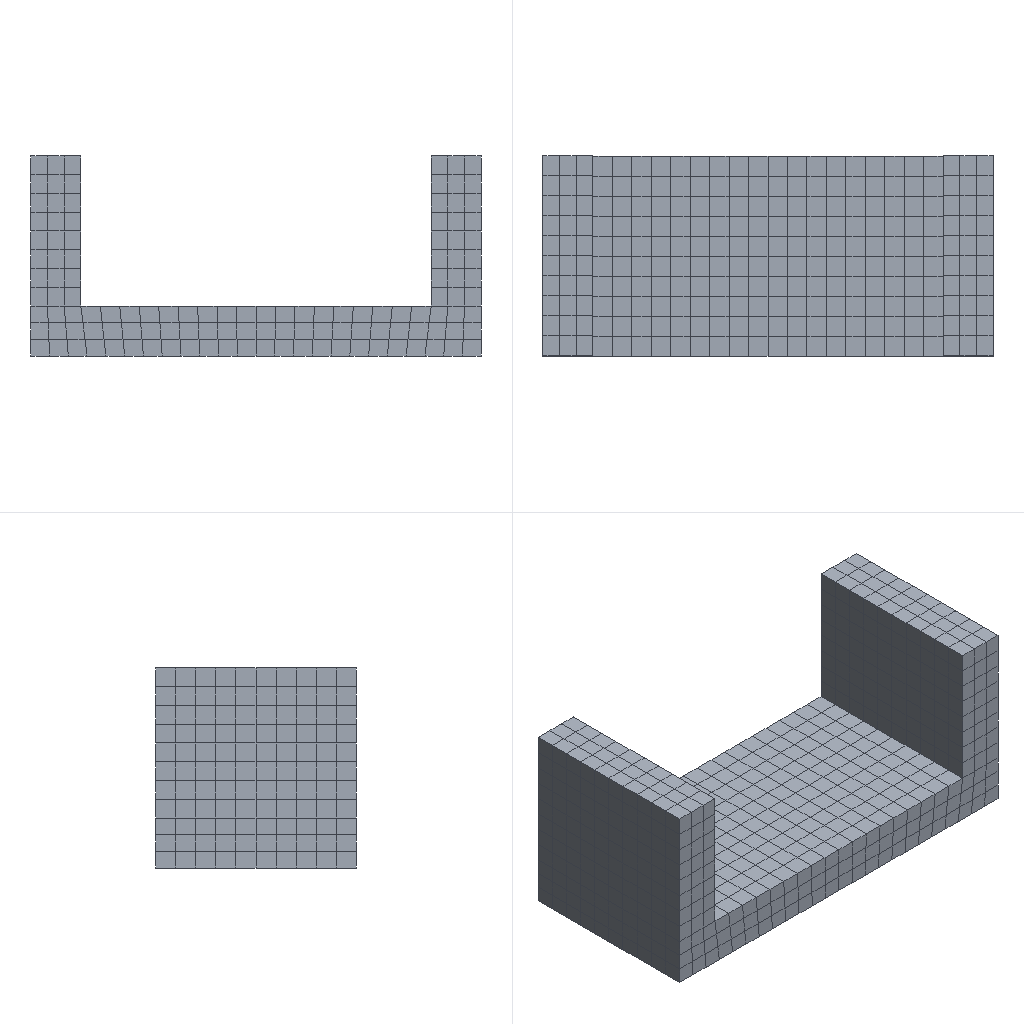Simulation study | abaqus
Notes in the study folder:
*Spring, elset=Springs/Dashpots-1-spring
1,1
 0.219E+06
*Element, type=Spring2, elset=Springs/Dashpots-1-spring
1,PART-1-1 .500001,PART-1-1 .2
*Spring, elset=Springs/Dashpots-2-spring
1,1
 0.219E+06
*Element, type=Spring2, elset=Springs/Dashpots-2-spring
2,PART-1-1 .500001,PART-1-1 .17
*Spring, elset=Springs/Dashpots-3-spring
1,1
 0.219E+06
*Element, type=Spring2, elset=Springs/Dashpots-3-spring
3,PART-1-1 .500002,PART-1-1 .3
*Spring, elset=Springs/Dashpots-4-spring
1,1
 0.219E+06
*Element, type=Spring2, elset=Springs/Dashpots-4-spring
4,PART-1-1 .500002,PART-1-1 .18
*Spring, elset=Springs/Dashpots-5-spring
1,1
 0.219E+06
*Element, type=Spring2, elset=Springs/Dashpots-5-spring
5,PART-1-1 .500003,PART-1-1 .36
*Spring, elset=Springs/Dashpots-6-spring
1,1
 0.219E+06
*Element, type=Spring2, elset=Springs/Dashpots-6-spring
6,PART-1-1 .500003,PART-1-1 .235
*Spring, elset=Springs/Dashpots-7-spring
1,1
 0.219E+06
*Element, type=Spring2, elset=Springs/Dashpots-7-spring
7,PART-1-1 .500004,PART-1-1 .35
*Spring, elset=Springs/Dashpots-8-spring
1,1
 0.219E+06
*Element, type=Spring2, elset=Springs/Dashpots-8-spring
8,PART-1-1 .500004,PART-1-1 .236
*Spring, elset=Springs/Dashpots-9-spring
1,1
 0.219E+06
*Element, type=Spring2, elset=Springs/Dashpots-9-spring
9,PART-1-1 .500005,PART-1-1 .34
*Spring, elset=Springs/Dashpots-10-spring
1,1
 0.219E+06
*Element, type=Spring2, elset=Springs/Dashpots-10-spring
10,PART-1-1 .500005,PART-1-1 .237
*Spring, elset=Springs/Dashpots-11-spring
1,1
 0.219E+06
*Element, type=Spring2, elset=Springs/Dashpots-11-spring
11,PART-1-1 .500006,PART-1-1 .33
*Spring, elset=Springs/Dashpots-12-spring
1,1
 0.219E+06
*Element, type=Spring2, elset=Springs/Dashpots-12-spring
12,PART-1-1 .500006,PART-1-1 .238
*Spring, elset=Springs/Dashpots-13-spring
1,1
 0.219E+06
*Element, type=Spring2, elset=Springs/Dashpots-13-spring
13,PART-1-1 .500007,PART-1-1 .32
*Spring, elset=Springs/Dashpots-14-spring
1,1
 0.219E+06
*Element, type=Spring2, elset=Springs/Dashpots-14-spring
14,PART-1-1 .500007,PART-1-1 .239
*Spring, elset=Springs/Dashpots-15-spring
1,1
 0.219E+06
*Element, type=Spring2, elset=Springs/Dashpots-15-spring
15,PART-1-1 .500008,PART-1-1 .31
*Spring, elset=Springs/Dashpots-16-spring
1,1
 0.219E+06
*Element, type=Spring2, elset=Springs/Dashpots-16-spring
16,PART-1-1 .500008,PART-1-1 .240
*Spring, elset=Springs/Dashpots-17-spring
1,1
 0.219E+06
*Element, type=Spring2, elset=Springs/Dashpots-17-spring
17,PART-1-1 .500009,PART-1-1 .30
*Spring, elset=Springs/Dashpots-18-spring
1,1
 0.219E+06
*Element, type=Spring2, elset=Springs/Dashpots-18-spring
18,PART-1-1 .500009,PART-1-1 .241
*Spring, elset=Springs/Dashpots-19-spring
1,1
 0.219E+06
*Element, type=Spring2, elset=Springs/Dashpots-19-spring
19,PART-1-1 .500010,PART-1-1 .29
*Spring, elset=Springs/Dashpots-20-spring
1,1
 0.219E+06
*Element, type=Spring2, elset=Springs/Dashpots-20-spring
20,PART-1-1 .500010,PART-1-1 .242
*Spring, elset=Springs/Dashpots-21-spring
1,1
 0.219E+06
*Element, type=Spring2, elset=Springs/Dashpots-21-spring
21,PART-1-1 .500011,PART-1-1 .28
*Spring, elset=Springs/Dashpots-22-spring
1,1
 0.219E+06
*Element, type=Spring2, elset=Springs/Dashpots-22-spring
22,PART-1-1 .500011,PART-1-1 .243
Set-up summary:
category,name,step,type,value,unit,region
solver,abaqus
solver,version,,,Abaqus/Standard 3DEXPERIENCE R2017x
units,not stated in the deck,,not stated
analysis,deck,,transient,transient
load_step,Step-1,Step-1,transient
load_step,requested,,,1
mesh,nodes,,,1804
mesh,elements,,,1200
element_type,C3D8R,,solid,1200
load,load commands in deck,,count,1
bc,support commands in deck,,count,3
material,MATERIAL-1,,in results
check,setup vs results,,match,"per instance, exact: element labels, types and connectivity; labels of the nodes the elements use; coordinates of those nodes at SINGLE_PRECISION in 1 of 1 instance(s)"
Abaqus input file, long lists of numbers shortened:
*Heading
** Job name: Job-1 Model name: Model-1
** Generated by: Abaqus/CAE 2017
*Preprint, echo=NO, model=NO, history=NO, contact=NO
**
** PARTS
**
*Part, name=Part-1
*End Part
**
**
** ASSEMBLY
**
*Assembly, name=Assembly
**
*Instance, name=Part-1-1, part=Part-1
          0.,          20.,           0.
          0.,          20.,           0.,           1.,          20.,           0.,          90.
*Node
      1,          40.,           5.,          20.
      2,          40.,          20.,          20.
** (1802 more lines like these left out)
*Element, type=C3D8R
  1,   87,  433, 1139,  397,    1,   21,  271,   52
  2,  433,  434, 1140, 1139,   21,   22,  272,  271
** (1198 more lines like these left out)
*Nset, nset=Set-1, generate
    1,  1804,     1
*Elset, elset=Set-1, generate
    1,  1200,     1
** Section: Section-1
*Solid Section, elset=Set-1, material=Material-1
,
*End Instance
**
*Nset, nset=Set-3, instance=Part-1-1
   15,   16,   17,   18,  212,  213,  214,  215,  216,  217,  218,  219,  220,  221,  222,  223
  224,  225,  226,  227,  228,  229,  230,  231,  232,  233,  234,  235,  236,  237,  238,  239
** (5 more lines like these left out)
*Elset, elset=Set-3, instance=Part-1-1, generate
  961,  1040,     1
*Nset, nset=Set-6, instance=Part-1-1
  11,  12,  13,  14, 104, 105, 106, 107, 108, 109, 110, 111, 112, 117, 118, 119
 120, 121, 122, 123, 124, 125, 128, 129, 130, 131, 132, 133, 134, 135, 136, 137
** (16 more lines like these left out)
*Elset, elset=Set-6, instance=Part-1-1
 261, 262, 263, 264, 265, 266, 267, 268, 269, 270, 291, 292, 293, 294, 295, 296
 297, 298, 299, 300, 321, 322, 323, 324, 325, 326, 327, 328, 329, 330, 351, 352
** (13 more lines like these left out)
*Nset, nset=Set-7, instance=Part-1-1
  11,  12,  13,  14, 104, 105, 106, 107, 108, 109, 110, 111, 112, 117, 118, 119
 120, 121, 122, 123, 124, 125, 128, 129, 130, 131, 132, 133, 134, 135, 136, 137
** (16 more lines like these left out)
*Elset, elset=Set-7, instance=Part-1-1
 261, 262, 263, 264, 265, 266, 267, 268, 269, 270, 291, 292, 293, 294, 295, 296
 297, 298, 299, 300, 321, 322, 323, 324, 325, 326, 327, 328, 329, 330, 351, 352
** (13 more lines like these left out)
*Nset, nset=c1, instance=Part-1-1
   15,   16,   17,   18,  212,  213,  214,  215,  216,  217,  218,  219,  220,  221,  222,  223
  224,  225,  226,  227,  228,  229,  230,  231,  232,  233,  234,  235,  236,  237,  238,  239
** (5 more lines like these left out)
*Nset, nset=c2, instance=Part-1-1
   1,   2,   3,   4,  21,  22,  23,  24,  25,  26,  27,  28,  29,  30,  31,  32
  33,  34,  35,  36,  37,  38,  39,  40,  41,  42,  43,  44,  45,  46,  47,  48
** (5 more lines like these left out)
*Nset, nset=di, instance=Part-1-1
   1,   4,  15,  16,  44,  45,  46,  47,  48,  49,  50,  51,  52, 153, 154, 155
 156, 157, 158, 159, 160, 161, 162, 163, 164, 165, 166, 167, 168, 169, 195, 196
** (12 more lines like these left out)
*Elset, elset=_Surf-1_S2, internal, instance=Part-1-1
    1,    2,    3,    4,    5,    6,    7,    8,    9,   10,   11,   12,   13,   14,   15,   16
   17,   18,   19,   20,   21,   22,   23,   24,   25,   26,   27,   28,   29,   30,   31,   32
** (8 more lines like these left out)
*Surface, type=ELEMENT, name=Surf-1
_Surf-1_S2, S2
*Elset, elset=_Surf-2_S3, internal, instance=Part-1-1
 331, 332, 333, 334, 335, 336, 337, 338, 339, 340, 361, 362, 363, 364, 365, 366
 367, 368, 369, 370, 391, 392, 393, 394, 395, 396, 397, 398, 399, 400, 421, 422
** (10 more lines like these left out)
*Surface, type=ELEMENT, name=Surf-2
_Surf-2_S3, S3
*Elset, elset=_Surf-3_S2, internal, instance=Part-1-1, generate
  961,  1040,     1
*Surface, type=ELEMENT, name=Surf-3
_Surf-3_S2, S2
*Elset, elset=_Surf-4_S2, internal, instance=Part-1-1, generate
  961,  1040,     1
*Surface, type=ELEMENT, name=Surf-4
_Surf-4_S2, S2
*Elset, elset=_Surf-5_S2, internal, instance=Part-1-1, generate
  1,  80,   1
*Surface, type=ELEMENT, name=Surf-5
_Surf-5_S2, S2
*Elset, elset=_Surf-6_S3, internal, instance=Part-1-1
 331, 332, 333, 334, 335, 336, 337, 338, 339, 340, 361, 362, 363, 364, 365, 366
 367, 368, 369, 370, 391, 392, 393, 394, 395, 396, 397, 398, 399, 400, 421, 422
** (10 more lines like these left out)
*Surface, type=ELEMENT, name=Surf-6
_Surf-6_S3, S3
*End Assembly
*Amplitude, name=Amp-1
             0.,              0.,            0.01,     0.09983,            0.02,     0.1987,            0.03,     0.2955
           0.04,     0.3894,            0.05,     0.4794,            0.06,     0.5646,            0.07,     0.6442
           0.08,     0.7174,            0.09,      0.7833,             0.1,     0.8415,            0.11,      0.8912
           0.12,     0.932,            0.13,     0.9636,            0.14,      0.9854,            0.15,     0.9975
           0.16,     0.9996,            0.17,      0.9917,            0.18,     0.9738,            0.19,     0.9463
            0.2,     0.9093,            0.21,     0.8632,            0.22,     0.8085,            0.23,     0.7457
           0.24,     0.6755,            0.25,     0.5985,            0.26,     0.5155,            0.27,      0.4274
           0.28,      0.335,            0.29,     0.2392,             0.3,     0.1411,            0.31,     0.04158
           0.32,    -0.05837,            0.33,    -0.1577,            0.34,    -0.2555,            0.35,    -0.3508
           0.36,    -0.4425,            0.37,    -0.5298,            0.38,    -0.6119,            0.39,    -0.6878
            0.4,    -0.7568,            0.41,    -0.8183,            0.42,    -0.8716,            0.43,    -0.9162
           0.44,    -0.9516,            0.45,    -0.9775,            0.46,    -0.9937,            0.47,    -0.9999
           0.48,    -0.9962,            0.49,    -0.9825,             0.5,    -0.9589,            0.51,    -0.9258
           0.52,    -0.8835,            0.53,    -0.8323,            0.54,    -0.7728,            0.55,    -0.7055
           0.56,    -0.6313,            0.57,    -0.5507,            0.58,    -0.4646,            0.59,    -0.3739
            0.6,    -0.2794,            0.61,    -0.1822,            0.62,    -0.08309,            0.63,       0.01681
           0.64,     0.1165,            0.65,     0.2151,            0.66,     0.3115,            0.67,     0.4048
           0.68,     0.4941,            0.69,     0.5784,             0.7,     0.657,            0.71,      0.729
           0.72,     0.7937,            0.73,     0.8504,            0.74,     0.8987,            0.75,     0.938
           0.76,     0.9679,            0.77,     0.9882,            0.78,     0.9985,            0.79,     0.9989
            0.8,     0.9894,            0.81,     0.9699,            0.82,     0.9407,            0.83,     0.9022
           0.84,     0.8546,            0.85,     0.7985,            0.86,     0.7344,            0.87,      0.663
           0.88,     0.5849,            0.89,     0.501,             0.9,     0.4121,            0.91,     0.3191
           0.92,     0.2229,            0.93,     0.1245,            0.94,     0.02478,            0.95,     -0.07515
           0.96,    -0.1743,            0.97,    -0.2718,            0.98,    -0.3665,            0.99,    -0.4575
             1.,    -0.544
**
** MATERIALS
**
*Material, name=Material-1
*Density
1000.,
*Elastic
 1e+10, 0.2
**
** BOUNDARY CONDITIONS
**
** Name: BC-2 Type: 位移/转角
*Boundary
Set-6, 2, 2
Set-6, 3, 3
** ----------------------------------------------------------------
**
** STEP: Step-1
**
*Step, name=Step-1, nlgeom=NO, inc=1000
*Dynamic
0.1,1.,1e-05
**
** BOUNDARY CONDITIONS
**
** Name: BC-3 Type: 加速度/角加速度
*Boundary, amplitude=Amp-1, type=ACCELERATION
Set-7, 1, 1, 1.
**
** OUTPUT REQUESTS
**
*Restart, write, frequency=0
**
** FIELD OUTPUT: F-Output-1
**
*Output, field, variable=PRESELECT, time interval=0.01
**
** HISTORY OUTPUT: H-Output-1
**
*Output, history, variable=PRESELECT, frequency=1
*End Step
Results summary:
result,step,,completed,increments=100 time=1.0/1.0
result,analysis,,,transient
result,last_loadstep,,,1
result,primary field,,,U
result,reaction total,,FX,-4340713.368,model units
result,reaction total,,FY,-0.0,model units
result,reaction total,,FZ,0.04326,model units